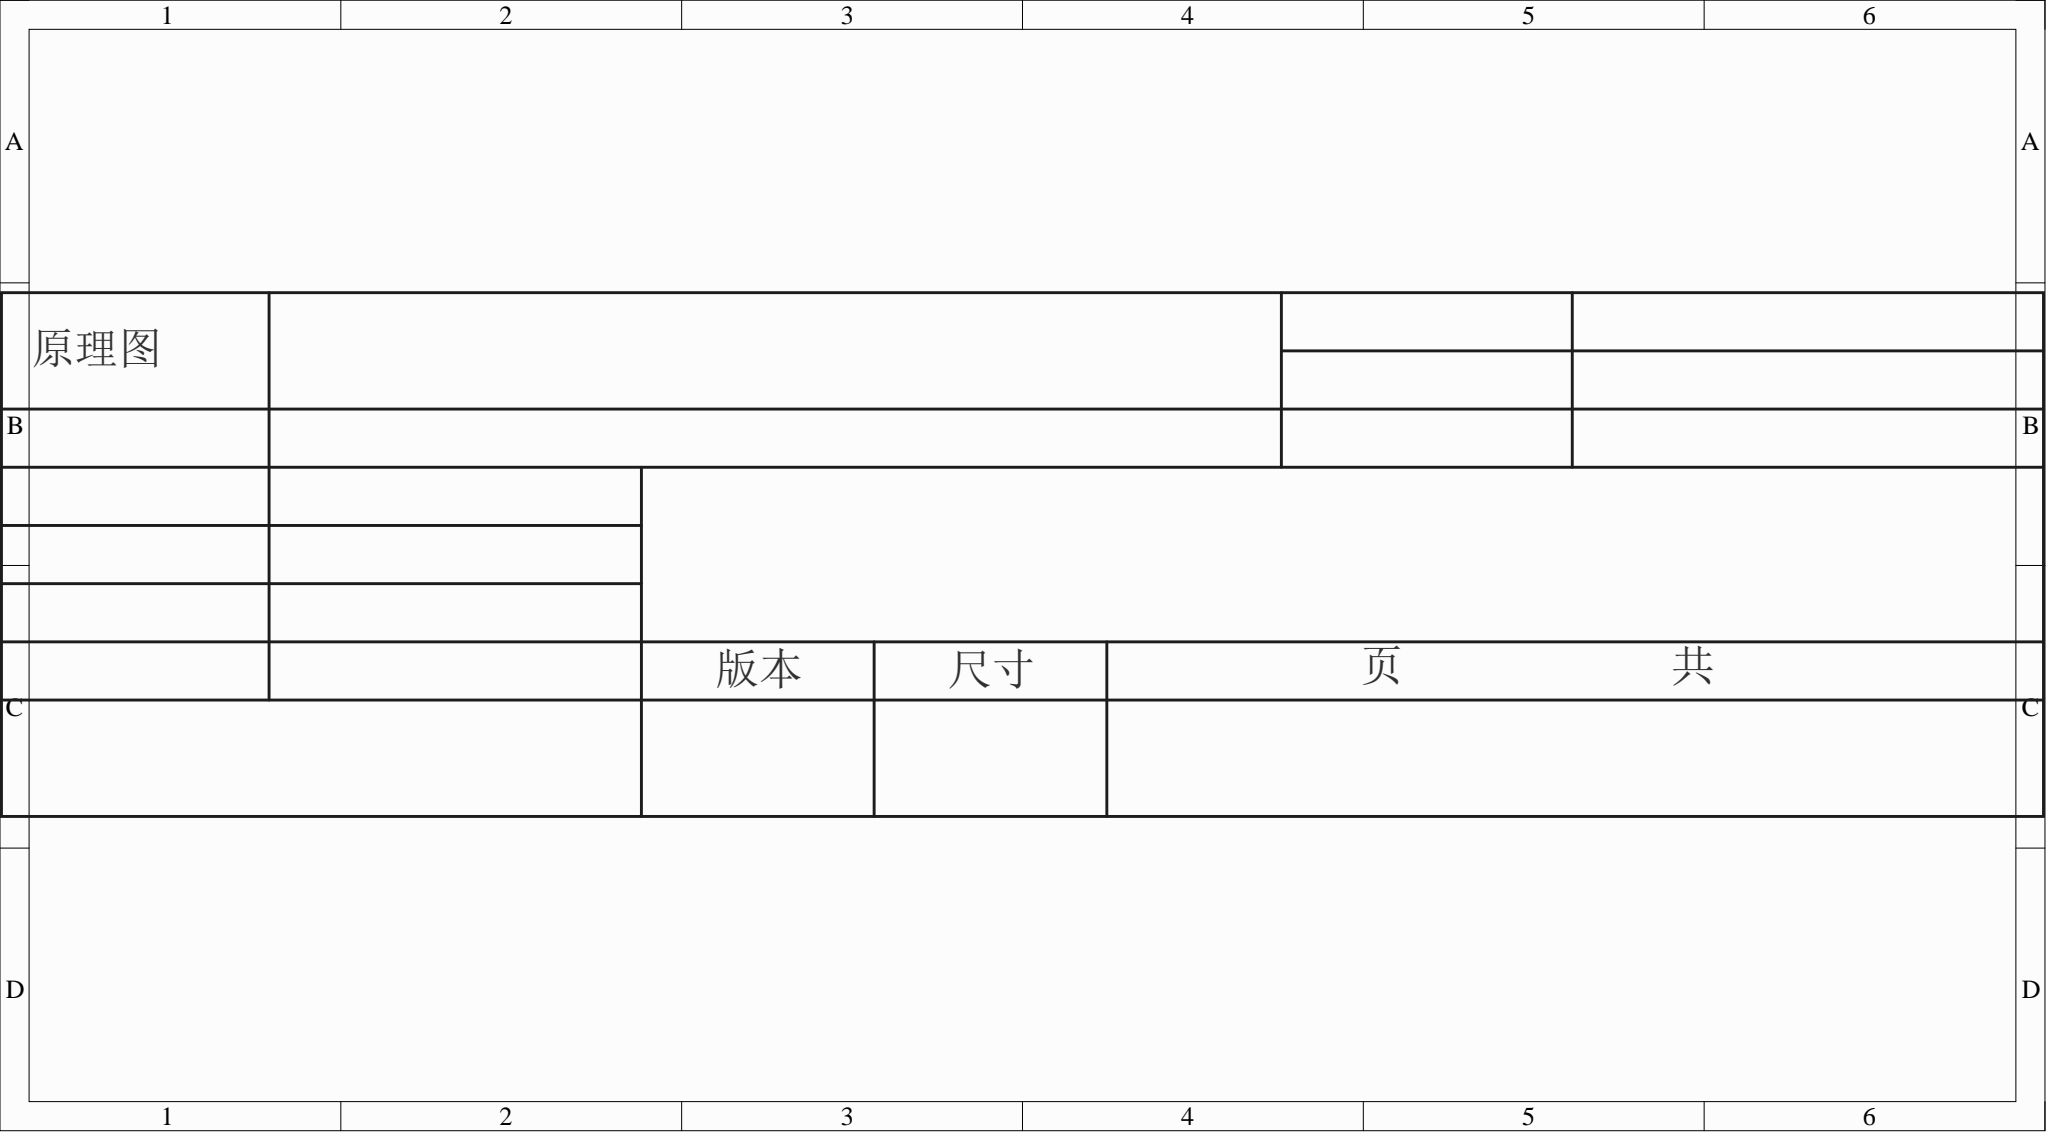Circuit board | Altium Designer | 70 parts | 124 nets
Bill of materials:
Comment,Description,Designator,Footprint,LibRef,Quantity
"1uF","","C1","C0805","CAP_0805","1"
"10nF","","C2","C0805","CAP_0805","1"
"","","H1","HDR-TH_2P-P2.54-V-M-1","HDR-M_2.54_1x2P","1"
"轻触按键3*4*H","","J8","SW-SMD_L4.0-W2.9-LS5.0","轻触按键3*4*H","1"
"","","LED5, LED7, LED11, LED12, LED13, LED14","LED-SEG-TH_10P-L12.6-W19.0-P2.54-S15.24-BL","LED_SEG_TH_0.56x1","6"
"10k","","R1","R0603","Res_0603","1"
"2.2k","","R2","R0603","Res_0603","1"
"250","","R44, R45, R46, R47, R48, R49, R50, R52, R53, R54, R55, R56, R57, R58, R61, R62, R63, R64, R65, R66, R67, R68, R69, R70, R71, R72, R73, R74, R75, R76, R77, R78, R79, R80, R81, R82, R83, R84, R85, R86, R87, R88","R0603","Res_0603","42"
"开关","","SW1","SW-TH_SS-12D01-GX","开关","1"
"NE555PE4","单精度计时器 8-PDIP 0 to 70","U8","PDIP-8_L9.6-W6.4-P2.54-LS7.9-BL-1","NE555PE4","1"
"SN74LS48N","","U70, U72, U79, U80, U83, U84","DIP-16_L19.3-W6.4-P2.54-LS7.6-BL","SN74LS48N","6"
"SN74LS08DR(LX)","逻辑类型:与门;通道数:4;电源电压:2V~6V;静态电流(最大值):2uA;最大传播延迟:15ns@6V;","U85","SOIC-14_L8.7-W3.9-P1.27-LS6.0-BL","SN74LS08DR(LX)","1"
"SN74LS00N(LX)","逻辑类型:与非门;通道数:4;电源电压:2V~6V;静态电流(最大值):2uA;最大传播延迟:7ns@6V;","U86","PDIP-14_L19.3-W6.4-P2.54-LS7.9-BL","SN74LS00N(LX)","1"
"SN74LS160N(LX)","工作电压:2V~6V;触发沿:上升沿;计数速率:35MHz;","U92, U93, U94, U95, U96, U97","DIP-16_L19.4-W6.4-P2.54-S7.6-BL","SN74LS160N(LX)","6"
Netlist (Protel format):
[
C1
C0805
1uF



]
[
C2
C0805
10nF



]
[
H1
HDR-TH_2P-P2.54-V-M-1




]
[
J8
SW-SMD_L4.0-W2.9-LS5.0
轻触按键3*4*H



]
[
LED5
LED-SEG-TH_10P-L12.6-W19.0-P2.54-S15.24-BL




]
[
LED7
LED-SEG-TH_10P-L12.6-W19.0-P2.54-S15.24-BL




]
[
LED11
LED-SEG-TH_10P-L12.6-W19.0-P2.54-S15.24-BL




]
[
LED12
LED-SEG-TH_10P-L12.6-W19.0-P2.54-S15.24-BL




]
[
LED13
LED-SEG-TH_10P-L12.6-W19.0-P2.54-S15.24-BL




]
[
LED14
LED-SEG-TH_10P-L12.6-W19.0-P2.54-S15.24-BL




]
[
R1
R0603
10k



]
[
R2
R0603
2.2k



]
[
R44
R0603
250



]
[
R45
R0603
250



]
[
R46
R0603
250



]
[
R47
R0603
250



]
[
R48
R0603
250



]
[
R49
R0603
250



]
[
R50
R0603
250



]
[
R52
R0603
250



]
[
R53
R0603
250



]
[
R54
R0603
250



]
[
R55
R0603
250



]
[
R56
R0603
250



]
[
R57
R0603
250



]
[
R58
R0603
250



]
[
R61
R0603
250



]
[
R62
R0603
250



]
[
R63
R0603
250



]
[
R64
R0603
250



]
[
R65
R0603
250



]
[
R66
R0603
250



]
[
R67
R0603
250



]
[
R68
R0603
250



]
[
R69
R0603
250



]
[
R70
R0603
250



]
[
R71
R0603
250



]
[
R72
R0603
250



]
[
R73
R0603
250



]
[
R74
R0603
250



]
[
R75
R0603
250



]
[
R76
R0603
250



]
[
R77
R0603
250



]
[
R78
R0603
250



]
[
R79
R0603
250



]
[
R80
R0603
250



]
[
R81
R0603
250



]
[
R82
R0603
250



]
[
R83
R0603
250



]
[
R84
R0603
250



]
[
R85
R0603
250



]
[
R86
R0603
250



]
[
R87
R0603
250



]
[
R88
R0603
250



]
[
SW1
SW-TH_SS-12D01-GX
开关



]
[
U8
PDIP-8_L9.6-W6.4-P2.54-LS7.9-BL-1
NE555PE4



]
[
U70
DIP-16_L19.3-W6.4-P2.54-LS7.6-BL
SN74LS48N



]
[
U72
DIP-16_L19.3-W6.4-P2.54-LS7.6-BL
SN74LS48N



]
[
U79
DIP-16_L19.3-W6.4-P2.54-LS7.6-BL
SN74LS48N



]
[
U80
DIP-16_L19.3-W6.4-P2.54-LS7.6-BL
SN74LS48N



]
[
U83
DIP-16_L19.3-W6.4-P2.54-LS7.6-BL
SN74LS48N



]
[
U84
DIP-16_L19.3-W6.4-P2.54-LS7.6-BL
SN74LS48N



]
[
U85
SOIC-14_L8.7-W3.9-P1.27-LS6.0-BL
SN74LS08DR(LX)



]
[
U86
PDIP-14_L19.3-W6.4-P2.54-LS7.9-BL
SN74LS00N(LX)



]
[
U92
DIP-16_L19.4-W6.4-P2.54-S7.6-BL
SN74LS160N(LX)



]
[
U93
DIP-16_L19.4-W6.4-P2.54-S7.6-BL
SN74LS160N(LX)



]
[
U94
DIP-16_L19.4-W6.4-P2.54-S7.6-BL
SN74LS160N(LX)



]
[
U95
DIP-16_L19.4-W6.4-P2.54-S7.6-BL
SN74LS160N(LX)



]
[
U96
DIP-16_L19.4-W6.4-P2.54-S7.6-BL
SN74LS160N(LX)



]
[
U97
DIP-16_L19.4-W6.4-P2.54-S7.6-BL
SN74LS160N(LX)



]
(
VCC
H1-1
R1-2
SW1-1
U8-4
U8-8
U70-3
U70-4
U70-5
U70-16
U72-3
U72-4
U72-5
U72-16
U79-3
U79-4
U79-5
U79-16
U80-3
U80-4
U80-5
U80-16
U83-3
U83-4
U83-5
U83-16
U84-3
U84-4
U84-5
U84-16
U85-14
U86-14
U92-7
U92-9
U92-10
U92-16
U93-7
U93-9
U93-10
U93-16
U94-7
U94-9
U94-10
U94-16
U95-7
U95-9
U95-10
U95-16
U96-7
U96-9
U96-10
U96-16
U97-7
U97-9
U97-10
U97-16
)
(
NetU96_2
U96-2
U97-15
)
(
NetU95_2
U95-2
U96-15
)
(
NetU94_2
U94-2
U95-15
)
(
NetU92_2
U92-2
U93-15
)
(
NetU85_10
U85-10
U86-8
)
(
NetU85_8
U85-8
U93-2
U94-1
)
(
NetU85_3
U85-3
U92-1
)
(
NetU85_2
U85-2
U86-6
)
(
NetU84_7
U84-7
U93-14
)
(
NetU84_6
U84-6
U93-11
)
(
NetU84_2
U84-2
U93-12
)
(
NetU84_1
U84-1
U93-13
)
(
NetU83_7
U83-7
U92-14
)
(
NetU83_6
U83-6
U92-11
)
(
NetU83_2
U83-2
U86-5
U92-12
)
(
NetU83_1
U83-1
U86-4
U92-13
)
(
NetU80_7
U80-7
U95-14
)
(
NetU80_6
U80-6
U95-11
)
(
NetU80_2
U80-2
U95-12
)
(
NetU80_1
U80-1
U95-13
)
(
NetU79_7
U79-7
U94-14
)
(
NetU79_6
U79-6
U94-11
)
(
NetU79_2
U79-2
U86-9
U94-12
)
(
NetU79_1
U79-1
U86-10
U94-13
)
(
NetU72_7
U72-7
U97-14
)
(
NetU72_6
U72-6
U97-11
)
(
NetU72_2
U72-2
U97-12
)
(
NetU72_1
U72-1
U97-13
)
(
NetU70_7
U70-7
U96-14
)
(
NetU70_6
U70-6
U96-11
)
(
NetU70_2
U70-2
U96-12
)
(
NetU70_1
U70-1
U96-13
)
(
NetSW1_2
SW1-2
U85-1
U85-9
U93-1
U95-1
U96-1
U97-1
)
(
NetR88_1
R88-1
U84-14
)
(
NetR87_1
R87-1
U84-15
)
(
NetR86_1
R86-1
U84-9
)
(
NetR85_1
R85-1
U84-10
)
(
NetR84_1
R84-1
U84-11
)
(
NetR83_1
R83-1
U84-12
)
(
NetR82_1
R82-1
U84-13
)
(
NetR81_1
R81-1
U83-14
)
(
NetR80_1
R80-1
U83-15
)
(
NetR79_1
R79-1
U83-9
)
(
NetR78_1
R78-1
U83-10
)
(
NetR77_1
R77-1
U83-11
)
(
NetR76_1
R76-1
U83-12
)
(
NetR75_1
R75-1
U83-13
)
(
NetR74_1
R74-1
U80-14
)
(
NetR73_1
R73-1
U80-15
)
(
NetR72_1
R72-1
U80-9
)
(
NetR71_1
R71-1
U80-10
)
(
NetR70_1
R70-1
U80-11
)
(
NetR69_1
R69-1
U80-12
)
(
NetR68_1
R68-1
U80-13
)
(
NetR67_1
R67-1
U79-14
)
(
NetR66_1
R66-1
U79-15
)
(
NetR65_1
R65-1
U79-9
)
(
NetR64_1
R64-1
U79-10
)
(
NetR63_1
R63-1
U79-11
)
(
NetR62_1
R62-1
U79-12
)
(
NetR61_1
R61-1
U79-13
)
(
NetR58_1
R58-1
U72-14
)
(
NetR57_1
R57-1
U72-15
)
(
NetR56_1
R56-1
U72-9
)
(
NetR55_1
R55-1
U72-10
)
(
NetR54_1
R54-1
U72-11
)
(
NetR53_1
R53-1
U72-12
)
(
NetR52_1
R52-1
U72-13
)
(
NetR50_1
R50-1
U70-14
)
(
NetR49_1
R49-1
U70-15
)
(
NetR48_1
R48-1
U70-9
)
(
NetR47_1
R47-1
U70-10
)
(
NetR46_1
R46-1
U70-11
)
(
NetR45_1
R45-1
U70-12
)
(
NetR44_1
R44-1
U70-13
)
(
NetR1_1
R1-1
R2-2
U8-7
)
(
NetLED14_10
LED14-10
R88-2
)
(
NetLED14_9
LED14-9
R87-2
)
(
NetLED14_7
LED14-7
R82-2
)
(
NetLED14_6
LED14-6
R83-2
)
(
NetLED14_4
LED14-4
R84-2
)
(
NetLED14_2
LED14-2
R85-2
)
(
NetLED14_1
LED14-1
R86-2
)
(
NetLED13_10
LED13-10
R81-2
)
(
NetLED13_9
LED13-9
R80-2
)
(
NetLED13_7
LED13-7
R75-2
)
(
NetLED13_6
LED13-6
R76-2
)
(
NetLED13_4
LED13-4
R77-2
)
(
NetLED13_2
LED13-2
R78-2
)
(
NetLED13_1
LED13-1
R79-2
)
(
NetLED12_10
LED12-10
R74-2
)
(
NetLED12_9
LED12-9
R73-2
)
(
NetLED12_7
LED12-7
R68-2
)
(
NetLED12_6
LED12-6
R69-2
)
(
NetLED12_4
LED12-4
R70-2
)
(
NetLED12_2
LED12-2
R71-2
)
(
NetLED12_1
LED12-1
R72-2
)
(
NetLED11_10
LED11-10
R67-2
)
(
NetLED11_9
LED11-9
R66-2
)
(
NetLED11_7
LED11-7
R61-2
)
(
NetLED11_6
LED11-6
R62-2
)
(
NetLED11_4
LED11-4
R63-2
)
(
NetLED11_2
LED11-2
R64-2
)
(
NetLED11_1
LED11-1
R65-2
)
(
NetLED7_10
LED7-10
R58-2
)
(
NetLED7_9
LED7-9
R57-2
)
(
NetLED7_7
LED7-7
R52-2
)
(
NetLED7_6
LED7-6
R53-2
)
(
NetLED7_4
LED7-4
R54-2
)
(
NetLED7_2
LED7-2
R55-2
)
(
NetLED7_1
LED7-1
R56-2
)
(
NetLED5_10
LED5-10
R50-2
)
(
NetLED5_9
LED5-9
R49-2
)
(
NetLED5_7
LED5-7
R44-2
)
(
NetLED5_6
LED5-6
R45-2
)
(
NetLED5_4
LED5-4
R46-2
)
(
NetLED5_2
LED5-2
R47-2
)
(
NetLED5_1
LED5-1
R48-2
)
(
NetJ8_2
J8-2
U97-2
)
(
NetJ8_1
J8-1
U8-3
)
(
NetC2_2
C2-2
U8-5
)
(
NetC1_2
C1-2
R2-1
U8-2
U8-6
)
(
GND
C1-1
C2-1
H1-2
LED5-3
LED5-8
LED7-3
LED7-8
LED11-3
LED11-8
LED12-3
LED12-8
LED13-3
LED13-8
LED14-3
LED14-8
SW1-3
U8-1
U70-8
U72-8
U79-8
U80-8
U83-8
U84-8
U85-7
U86-7
U92-3
U92-4
U92-5
U92-6
U92-8
U93-3
U93-4
U93-5
U93-6
U93-8
U94-3
U94-4
U94-5
U94-6
U94-8
U95-3
U95-4
U95-5
U95-6
U95-8
U96-3
U96-4
U96-5
U96-6
U96-8
U97-3
U97-4
U97-5
U97-6
U97-8
)